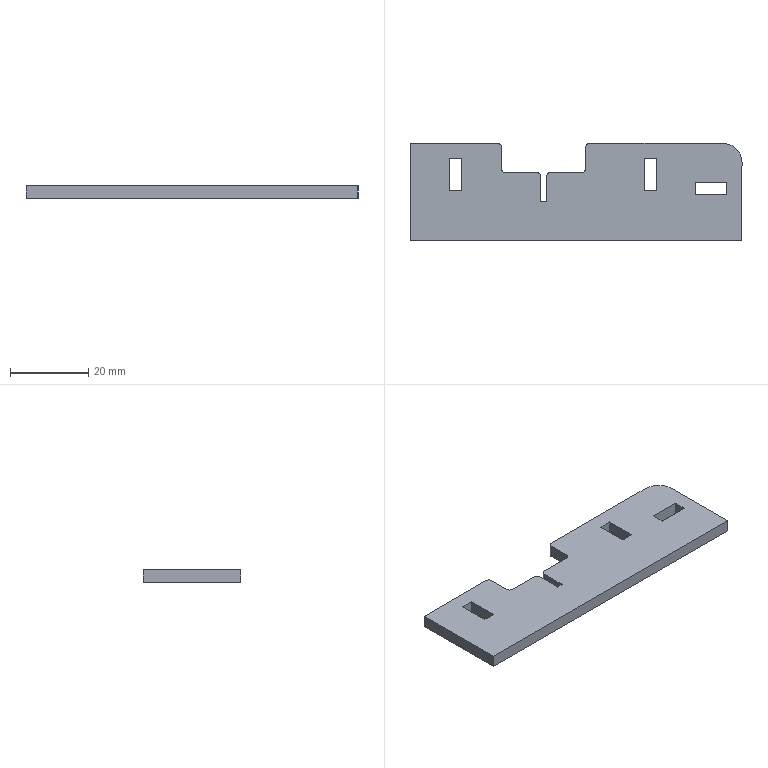Part | SolidWorks | features FlatPattern 1, SMBaseFlange 1, SheetMetal 1 | 1 solid | 33 faces | box 85 x 25 x 3.2 mm | volume 5979 mm3 | plane 26 | cylinder 7 | commonest cylinder face diameters 2 x6 10 x1
STEP:
#1=CARTESIAN_POINT('',(-85.,-5.,3.2));
#2=VERTEX_POINT('',#1);
#3=CARTESIAN_POINT('',(0.,-5.,3.2));
#4=VERTEX_POINT('',#3);
#5=CARTESIAN_POINT('',(0.,-5.,3.2));
#6=DIRECTION('',(1.,0.,0.));
#7=VECTOR('',#6,1000.);
#8=LINE('',#5,#7);
#9=EDGE_CURVE('',#2,#4,#8,.T.);
#10=ORIENTED_EDGE('',*,*,#9,.T.);
#11=CARTESIAN_POINT('',(0.,15.,3.2));
#12=VERTEX_POINT('',#11);
#13=CARTESIAN_POINT('',(0.,15.,3.2));
#14=DIRECTION('',(0.,1.,0.));
#15=VECTOR('',#14,1000.);
#16=LINE('',#13,#15);
#17=EDGE_CURVE('',#4,#12,#16,.T.);
#18=ORIENTED_EDGE('',*,*,#17,.T.);
#19=CARTESIAN_POINT('',(-5.,20.,3.2));
#20=VERTEX_POINT('',#19);
#21=CARTESIAN_POINT('',(-5.,15.,3.2));
#22=DIRECTION('',(0.,0.,1.));
#23=DIRECTION('',(-1.,0.,0.));
#24=AXIS2_PLACEMENT_3D('',#21,#22,#23);
#25=CIRCLE('',#24,5.);
#26=EDGE_CURVE('',#12,#20,#25,.T.);
#27=ORIENTED_EDGE('',*,*,#26,.T.);
#28=CARTESIAN_POINT('',(-39.,20.,3.2));
#29=VERTEX_POINT('',#28);
#30=CARTESIAN_POINT('',(-39.,20.,3.2));
#31=DIRECTION('',(-1.,0.,0.));
#32=VECTOR('',#31,1000.);
#33=LINE('',#30,#32);
#34=EDGE_CURVE('',#20,#29,#33,.T.);
#35=ORIENTED_EDGE('',*,*,#34,.T.);
#36=CARTESIAN_POINT('',(-40.,19.,3.2));
#37=VERTEX_POINT('',#36);
#38=CARTESIAN_POINT('',(-39.,19.,3.2));
#39=DIRECTION('',(0.,0.,1.));
#40=DIRECTION('',(-1.,0.,0.));
#41=AXIS2_PLACEMENT_3D('',#38,#39,#40);
#42=CIRCLE('',#41,1.);
#43=EDGE_CURVE('',#29,#37,#42,.T.);
#44=ORIENTED_EDGE('',*,*,#43,.T.);
#45=CARTESIAN_POINT('',(-40.,13.5,3.2));
#46=VERTEX_POINT('',#45);
#47=CARTESIAN_POINT('',(-40.,13.5,3.2));
#48=DIRECTION('',(0.,-1.,0.));
#49=VECTOR('',#48,1000.);
#50=LINE('',#47,#49);
#51=EDGE_CURVE('',#37,#46,#50,.T.);
#52=ORIENTED_EDGE('',*,*,#51,.T.);
#53=CARTESIAN_POINT('',(-41.,12.5,3.2));
#54=VERTEX_POINT('',#53);
#55=CARTESIAN_POINT('',(-41.,13.5,3.2));
#56=DIRECTION('',(0.,0.,-1.));
#57=DIRECTION('',(1.,0.,0.));
#58=AXIS2_PLACEMENT_3D('',#55,#56,#57);
#59=CIRCLE('',#58,1.);
#60=EDGE_CURVE('',#46,#54,#59,.T.);
#61=ORIENTED_EDGE('',*,*,#60,.T.);
#62=CARTESIAN_POINT('',(-49.,12.5,3.2));
#63=VERTEX_POINT('',#62);
#64=CARTESIAN_POINT('',(-49.,12.5,3.2));
#65=DIRECTION('',(-1.,0.,0.));
#66=VECTOR('',#65,1000.);
#67=LINE('',#64,#66);
#68=EDGE_CURVE('',#54,#63,#67,.T.);
#69=ORIENTED_EDGE('',*,*,#68,.T.);
#70=CARTESIAN_POINT('',(-50.,11.5,3.2));
#71=VERTEX_POINT('',#70);
#72=CARTESIAN_POINT('',(-49.,11.5,3.2));
#73=DIRECTION('',(0.,0.,1.));
#74=DIRECTION('',(1.,0.,0.));
#75=AXIS2_PLACEMENT_3D('',#72,#73,#74);
#76=CIRCLE('',#75,1.);
#77=EDGE_CURVE('',#63,#71,#76,.T.);
#78=ORIENTED_EDGE('',*,*,#77,.T.);
#79=CARTESIAN_POINT('',(-50.,5.,3.2));
#80=VERTEX_POINT('',#79);
#81=CARTESIAN_POINT('',(-50.,5.,3.2));
#82=DIRECTION('',(0.,-1.,0.));
#83=VECTOR('',#82,1000.);
#84=LINE('',#81,#83);
#85=EDGE_CURVE('',#71,#80,#84,.T.);
#86=ORIENTED_EDGE('',*,*,#85,.T.);
#87=CARTESIAN_POINT('',(-51.6,5.,3.2));
#88=VERTEX_POINT('',#87);
#89=CARTESIAN_POINT('',(-51.6,5.,3.2));
#90=DIRECTION('',(-1.,0.,0.));
#91=VECTOR('',#90,1000.);
#92=LINE('',#89,#91);
#93=EDGE_CURVE('',#80,#88,#92,.T.);
#94=ORIENTED_EDGE('',*,*,#93,.T.);
#95=CARTESIAN_POINT('',(-51.6,11.5,3.2));
#96=VERTEX_POINT('',#95);
#97=CARTESIAN_POINT('',(-51.6,11.5,3.2));
#98=DIRECTION('',(0.,1.,0.));
#99=VECTOR('',#98,1000.);
#100=LINE('',#97,#99);
#101=EDGE_CURVE('',#88,#96,#100,.T.);
#102=ORIENTED_EDGE('',*,*,#101,.T.);
#103=CARTESIAN_POINT('',(-52.6,12.5,3.2));
#104=VERTEX_POINT('',#103);
#105=CARTESIAN_POINT('',(-52.6,11.5,3.2));
#106=DIRECTION('',(0.,0.,1.));
#107=DIRECTION('',(-1.,0.,0.));
#108=AXIS2_PLACEMENT_3D('',#105,#106,#107);
#109=CIRCLE('',#108,1.);
#110=EDGE_CURVE('',#96,#104,#109,.T.);
#111=ORIENTED_EDGE('',*,*,#110,.T.);
#112=CARTESIAN_POINT('',(-60.6,12.5,3.2));
#113=VERTEX_POINT('',#112);
#114=CARTESIAN_POINT('',(-52.6,12.5,3.2));
#115=DIRECTION('',(-1.,0.,0.));
#116=VECTOR('',#115,1000.);
#117=LINE('',#114,#116);
#118=EDGE_CURVE('',#104,#113,#117,.T.);
#119=ORIENTED_EDGE('',*,*,#118,.T.);
#120=CARTESIAN_POINT('',(-61.6,13.5,3.2));
#121=VERTEX_POINT('',#120);
#122=CARTESIAN_POINT('',(-60.6,13.5,3.2));
#123=DIRECTION('',(0.,0.,-1.));
#124=DIRECTION('',(-1.,0.,0.));
#125=AXIS2_PLACEMENT_3D('',#122,#123,#124);
#126=CIRCLE('',#125,1.);
#127=EDGE_CURVE('',#113,#121,#126,.T.);
#128=ORIENTED_EDGE('',*,*,#127,.T.);
#129=CARTESIAN_POINT('',(-61.6,19.,3.2));
#130=VERTEX_POINT('',#129);
#131=CARTESIAN_POINT('',(-61.6,13.5,3.2));
#132=DIRECTION('',(0.,1.,0.));
#133=VECTOR('',#132,1000.);
#134=LINE('',#131,#133);
#135=EDGE_CURVE('',#121,#130,#134,.T.);
#136=ORIENTED_EDGE('',*,*,#135,.T.);
#137=CARTESIAN_POINT('',(-62.6,20.,3.2));
#138=VERTEX_POINT('',#137);
#139=CARTESIAN_POINT('',(-62.6,19.,3.2));
#140=DIRECTION('',(0.,0.,1.));
#141=DIRECTION('',(1.,0.,0.));
#142=AXIS2_PLACEMENT_3D('',#139,#140,#141);
#143=CIRCLE('',#142,1.);
#144=EDGE_CURVE('',#130,#138,#143,.T.);
#145=ORIENTED_EDGE('',*,*,#144,.T.);
#146=CARTESIAN_POINT('',(-85.,20.,3.2));
#147=VERTEX_POINT('',#146);
#148=CARTESIAN_POINT('',(-85.,20.,3.2));
#149=DIRECTION('',(-1.,0.,0.));
#150=VECTOR('',#149,1000.);
#151=LINE('',#148,#150);
#152=EDGE_CURVE('',#138,#147,#151,.T.);
#153=ORIENTED_EDGE('',*,*,#152,.T.);
#154=CARTESIAN_POINT('',(-85.,-5.,3.2));
#155=DIRECTION('',(0.,-1.,0.));
#156=VECTOR('',#155,1000.);
#157=LINE('',#154,#156);
#158=EDGE_CURVE('',#147,#2,#157,.T.);
#159=ORIENTED_EDGE('',*,*,#158,.T.);
#160=EDGE_LOOP('',(#10,#18,#27,#35,#44,#52,#61,#69,#78,#86,#94,#102,#111,#119,#128,#136,#145,#153,#159));
#161=FACE_OUTER_BOUND('',#160,.T.);
#162=CARTESIAN_POINT('',(-4.,10.,3.2));
#163=VERTEX_POINT('',#162);
#164=CARTESIAN_POINT('',(-12.,10.,3.2));
#165=VERTEX_POINT('',#164);
#166=CARTESIAN_POINT('',(-4.,10.,3.2));
#167=DIRECTION('',(-1.,0.,0.));
#168=VECTOR('',#167,1000.);
#169=LINE('',#166,#168);
#170=EDGE_CURVE('',#163,#165,#169,.T.);
#171=ORIENTED_EDGE('',*,*,#170,.F.);
#172=CARTESIAN_POINT('',(-4.,6.8,3.2));
#173=VERTEX_POINT('',#172);
#174=CARTESIAN_POINT('',(-4.,10.,3.2));
#175=DIRECTION('',(0.,1.,0.));
#176=VECTOR('',#175,1000.);
#177=LINE('',#174,#176);
#178=EDGE_CURVE('',#173,#163,#177,.T.);
#179=ORIENTED_EDGE('',*,*,#178,.F.);
#180=CARTESIAN_POINT('',(-12.,6.8,3.2));
#181=VERTEX_POINT('',#180);
#182=CARTESIAN_POINT('',(-4.,6.8,3.2));
#183=DIRECTION('',(1.,0.,0.));
#184=VECTOR('',#183,1000.);
#185=LINE('',#182,#184);
#186=EDGE_CURVE('',#181,#173,#185,.T.);
#187=ORIENTED_EDGE('',*,*,#186,.F.);
#188=CARTESIAN_POINT('',(-12.,10.,3.2));
#189=DIRECTION('',(0.,-1.,0.));
#190=VECTOR('',#189,1000.);
#191=LINE('',#188,#190);
#192=EDGE_CURVE('',#165,#181,#191,.T.);
#193=ORIENTED_EDGE('',*,*,#192,.F.);
#194=EDGE_LOOP('',(#171,#179,#187,#193));
#195=FACE_BOUND('',#194,.T.);
#196=CARTESIAN_POINT('',(-25.,8.,3.2));
#197=VERTEX_POINT('',#196);
#198=CARTESIAN_POINT('',(-21.8,8.,3.2));
#199=VERTEX_POINT('',#198);
#200=CARTESIAN_POINT('',(-25.,8.,3.2));
#201=DIRECTION('',(1.,0.,0.));
#202=VECTOR('',#201,1000.);
#203=LINE('',#200,#202);
#204=EDGE_CURVE('',#197,#199,#203,.T.);
#205=ORIENTED_EDGE('',*,*,#204,.F.);
#206=CARTESIAN_POINT('',(-25.,16.,3.2));
#207=VERTEX_POINT('',#206);
#208=CARTESIAN_POINT('',(-25.,8.,3.2));
#209=DIRECTION('',(0.,-1.,0.));
#210=VECTOR('',#209,1000.);
#211=LINE('',#208,#210);
#212=EDGE_CURVE('',#207,#197,#211,.T.);
#213=ORIENTED_EDGE('',*,*,#212,.F.);
#214=CARTESIAN_POINT('',(-21.8,16.,3.2));
#215=VERTEX_POINT('',#214);
#216=CARTESIAN_POINT('',(-25.,16.,3.2));
#217=DIRECTION('',(-1.,0.,0.));
#218=VECTOR('',#217,1000.);
#219=LINE('',#216,#218);
#220=EDGE_CURVE('',#215,#207,#219,.T.);
#221=ORIENTED_EDGE('',*,*,#220,.F.);
#222=CARTESIAN_POINT('',(-21.8,8.,3.2));
#223=DIRECTION('',(0.,1.,0.));
#224=VECTOR('',#223,1000.);
#225=LINE('',#222,#224);
#226=EDGE_CURVE('',#199,#215,#225,.T.);
#227=ORIENTED_EDGE('',*,*,#226,.F.);
#228=EDGE_LOOP('',(#205,#213,#221,#227));
#229=FACE_BOUND('',#228,.T.);
#230=CARTESIAN_POINT('',(-71.8,16.,3.2));
#231=VERTEX_POINT('',#230);
#232=CARTESIAN_POINT('',(-75.,16.,3.2));
#233=VERTEX_POINT('',#232);
#234=CARTESIAN_POINT('',(-71.8,16.,3.2));
#235=DIRECTION('',(-1.,0.,0.));
#236=VECTOR('',#235,1000.);
#237=LINE('',#234,#236);
#238=EDGE_CURVE('',#231,#233,#237,.T.);
#239=ORIENTED_EDGE('',*,*,#238,.F.);
#240=CARTESIAN_POINT('',(-71.8,8.,3.2));
#241=VERTEX_POINT('',#240);
#242=CARTESIAN_POINT('',(-71.8,8.,3.2));
#243=DIRECTION('',(0.,1.,0.));
#244=VECTOR('',#243,1000.);
#245=LINE('',#242,#244);
#246=EDGE_CURVE('',#241,#231,#245,.T.);
#247=ORIENTED_EDGE('',*,*,#246,.F.);
#248=CARTESIAN_POINT('',(-75.,8.,3.2));
#249=VERTEX_POINT('',#248);
#250=CARTESIAN_POINT('',(-71.8,8.,3.2));
#251=DIRECTION('',(1.,0.,0.));
#252=VECTOR('',#251,1000.);
#253=LINE('',#250,#252);
#254=EDGE_CURVE('',#249,#241,#253,.T.);
#255=ORIENTED_EDGE('',*,*,#254,.F.);
#256=CARTESIAN_POINT('',(-75.,8.,3.2));
#257=DIRECTION('',(0.,-1.,0.));
#258=VECTOR('',#257,1000.);
#259=LINE('',#256,#258);
#260=EDGE_CURVE('',#233,#249,#259,.T.);
#261=ORIENTED_EDGE('',*,*,#260,.F.);
#262=EDGE_LOOP('',(#239,#247,#255,#261));
#263=FACE_BOUND('',#262,.T.);
#264=CARTESIAN_POINT('',(-62.6,19.,3.2));
#265=DIRECTION('',(0.,0.,1.));
#266=DIRECTION('',(1.,0.,0.));
#267=AXIS2_PLACEMENT_3D('',#264,#265,#266);
#268=PLANE('',#267);
#269=ADVANCED_FACE('',(#161,#195,#229,#263),#268,.T.);
#270=CARTESIAN_POINT('',(-25.,16.,0.));
#271=VERTEX_POINT('',#270);
#272=CARTESIAN_POINT('',(-25.,8.,0.));
#273=VERTEX_POINT('',#272);
#274=CARTESIAN_POINT('',(-25.,8.,0.));
#275=DIRECTION('',(0.,-1.,0.));
#276=VECTOR('',#275,1000.);
#277=LINE('',#274,#276);
#278=EDGE_CURVE('',#271,#273,#277,.T.);
#279=ORIENTED_EDGE('',*,*,#278,.T.);
#280=CARTESIAN_POINT('',(-21.8,8.,0.));
#281=VERTEX_POINT('',#280);
#282=CARTESIAN_POINT('',(-25.,8.,0.));
#283=DIRECTION('',(1.,0.,0.));
#284=VECTOR('',#283,1000.);
#285=LINE('',#282,#284);
#286=EDGE_CURVE('',#273,#281,#285,.T.);
#287=ORIENTED_EDGE('',*,*,#286,.T.);
#288=CARTESIAN_POINT('',(-21.8,16.,0.));
#289=VERTEX_POINT('',#288);
#290=CARTESIAN_POINT('',(-21.8,8.,0.));
#291=DIRECTION('',(0.,1.,0.));
#292=VECTOR('',#291,1000.);
#293=LINE('',#290,#292);
#294=EDGE_CURVE('',#281,#289,#293,.T.);
#295=ORIENTED_EDGE('',*,*,#294,.T.);
#296=CARTESIAN_POINT('',(-25.,16.,0.));
#297=DIRECTION('',(-1.,0.,0.));
#298=VECTOR('',#297,1000.);
#299=LINE('',#296,#298);
#300=EDGE_CURVE('',#289,#271,#299,.T.);
#301=ORIENTED_EDGE('',*,*,#300,.T.);
#302=EDGE_LOOP('',(#279,#287,#295,#301));
#303=FACE_BOUND('',#302,.T.);
#304=CARTESIAN_POINT('',(-85.,-5.,0.));
#305=VERTEX_POINT('',#304);
#306=CARTESIAN_POINT('',(0.,-5.,0.));
#307=VERTEX_POINT('',#306);
#308=CARTESIAN_POINT('',(0.,-5.,0.));
#309=DIRECTION('',(1.,0.,0.));
#310=VECTOR('',#309,1000.);
#311=LINE('',#308,#310);
#312=EDGE_CURVE('',#305,#307,#311,.T.);
#313=ORIENTED_EDGE('',*,*,#312,.F.);
#314=CARTESIAN_POINT('',(-85.,20.,0.));
#315=VERTEX_POINT('',#314);
#316=CARTESIAN_POINT('',(-85.,-5.,0.));
#317=DIRECTION('',(0.,-1.,0.));
#318=VECTOR('',#317,1000.);
#319=LINE('',#316,#318);
#320=EDGE_CURVE('',#315,#305,#319,.T.);
#321=ORIENTED_EDGE('',*,*,#320,.F.);
#322=CARTESIAN_POINT('',(-62.6,20.,0.));
#323=VERTEX_POINT('',#322);
#324=CARTESIAN_POINT('',(-85.,20.,0.));
#325=DIRECTION('',(-1.,0.,0.));
#326=VECTOR('',#325,1000.);
#327=LINE('',#324,#326);
#328=EDGE_CURVE('',#323,#315,#327,.T.);
#329=ORIENTED_EDGE('',*,*,#328,.F.);
#330=CARTESIAN_POINT('',(-61.6,19.,0.));
#331=VERTEX_POINT('',#330);
#332=CARTESIAN_POINT('',(-62.6,19.,0.));
#333=DIRECTION('',(0.,0.,1.));
#334=DIRECTION('',(1.,0.,0.));
#335=AXIS2_PLACEMENT_3D('',#332,#333,#334);
#336=CIRCLE('',#335,1.);
#337=EDGE_CURVE('',#331,#323,#336,.T.);
#338=ORIENTED_EDGE('',*,*,#337,.F.);
#339=CARTESIAN_POINT('',(-61.6,13.5,0.));
#340=VERTEX_POINT('',#339);
#341=CARTESIAN_POINT('',(-61.6,13.5,0.));
#342=DIRECTION('',(0.,1.,0.));
#343=VECTOR('',#342,1000.);
#344=LINE('',#341,#343);
#345=EDGE_CURVE('',#340,#331,#344,.T.);
#346=ORIENTED_EDGE('',*,*,#345,.F.);
#347=CARTESIAN_POINT('',(-60.6,12.5,0.));
#348=VERTEX_POINT('',#347);
#349=CARTESIAN_POINT('',(-60.6,13.5,0.));
#350=DIRECTION('',(0.,0.,-1.));
#351=DIRECTION('',(-1.,0.,0.));
#352=AXIS2_PLACEMENT_3D('',#349,#350,#351);
#353=CIRCLE('',#352,1.);
#354=EDGE_CURVE('',#348,#340,#353,.T.);
#355=ORIENTED_EDGE('',*,*,#354,.F.);
#356=CARTESIAN_POINT('',(-52.6,12.5,0.));
#357=VERTEX_POINT('',#356);
#358=CARTESIAN_POINT('',(-52.6,12.5,0.));
#359=DIRECTION('',(-1.,0.,0.));
#360=VECTOR('',#359,1000.);
#361=LINE('',#358,#360);
#362=EDGE_CURVE('',#357,#348,#361,.T.);
#363=ORIENTED_EDGE('',*,*,#362,.F.);
#364=CARTESIAN_POINT('',(-51.6,11.5,0.));
#365=VERTEX_POINT('',#364);
#366=CARTESIAN_POINT('',(-52.6,11.5,0.));
#367=DIRECTION('',(0.,0.,1.));
#368=DIRECTION('',(-1.,0.,0.));
#369=AXIS2_PLACEMENT_3D('',#366,#367,#368);
#370=CIRCLE('',#369,1.);
#371=EDGE_CURVE('',#365,#357,#370,.T.);
#372=ORIENTED_EDGE('',*,*,#371,.F.);
#373=CARTESIAN_POINT('',(-51.6,5.,0.));
#374=VERTEX_POINT('',#373);
#375=CARTESIAN_POINT('',(-51.6,11.5,0.));
#376=DIRECTION('',(0.,1.,0.));
#377=VECTOR('',#376,1000.);
#378=LINE('',#375,#377);
#379=EDGE_CURVE('',#374,#365,#378,.T.);
#380=ORIENTED_EDGE('',*,*,#379,.F.);
#381=CARTESIAN_POINT('',(-50.,5.,0.));
#382=VERTEX_POINT('',#381);
#383=CARTESIAN_POINT('',(-51.6,5.,0.));
#384=DIRECTION('',(-1.,0.,0.));
#385=VECTOR('',#384,1000.);
#386=LINE('',#383,#385);
#387=EDGE_CURVE('',#382,#374,#386,.T.);
#388=ORIENTED_EDGE('',*,*,#387,.F.);
#389=CARTESIAN_POINT('',(-50.,11.5,0.));
#390=VERTEX_POINT('',#389);
#391=CARTESIAN_POINT('',(-50.,5.,0.));
#392=DIRECTION('',(0.,-1.,0.));
#393=VECTOR('',#392,1000.);
#394=LINE('',#391,#393);
#395=EDGE_CURVE('',#390,#382,#394,.T.);
#396=ORIENTED_EDGE('',*,*,#395,.F.);
#397=CARTESIAN_POINT('',(-49.,12.5,0.));
#398=VERTEX_POINT('',#397);
#399=CARTESIAN_POINT('',(-49.,11.5,0.));
#400=DIRECTION('',(0.,0.,1.));
#401=DIRECTION('',(1.,0.,0.));
#402=AXIS2_PLACEMENT_3D('',#399,#400,#401);
#403=CIRCLE('',#402,1.);
#404=EDGE_CURVE('',#398,#390,#403,.T.);
#405=ORIENTED_EDGE('',*,*,#404,.F.);
#406=CARTESIAN_POINT('',(-41.,12.5,0.));
#407=VERTEX_POINT('',#406);
#408=CARTESIAN_POINT('',(-49.,12.5,0.));
#409=DIRECTION('',(-1.,0.,0.));
#410=VECTOR('',#409,1000.);
#411=LINE('',#408,#410);
#412=EDGE_CURVE('',#407,#398,#411,.T.);
#413=ORIENTED_EDGE('',*,*,#412,.F.);
#414=CARTESIAN_POINT('',(-40.,13.5,0.));
#415=VERTEX_POINT('',#414);
#416=CARTESIAN_POINT('',(-41.,13.5,0.));
#417=DIRECTION('',(0.,0.,-1.));
#418=DIRECTION('',(1.,0.,0.));
#419=AXIS2_PLACEMENT_3D('',#416,#417,#418);
#420=CIRCLE('',#419,1.);
#421=EDGE_CURVE('',#415,#407,#420,.T.);
#422=ORIENTED_EDGE('',*,*,#421,.F.);
#423=CARTESIAN_POINT('',(-40.,19.,0.));
#424=VERTEX_POINT('',#423);
#425=CARTESIAN_POINT('',(-40.,13.5,0.));
#426=DIRECTION('',(0.,-1.,0.));
#427=VECTOR('',#426,1000.);
#428=LINE('',#425,#427);
#429=EDGE_CURVE('',#424,#415,#428,.T.);
#430=ORIENTED_EDGE('',*,*,#429,.F.);
#431=CARTESIAN_POINT('',(-39.,20.,0.));
#432=VERTEX_POINT('',#431);
#433=CARTESIAN_POINT('',(-39.,19.,0.));
#434=DIRECTION('',(0.,0.,1.));
#435=DIRECTION('',(-1.,0.,0.));
#436=AXIS2_PLACEMENT_3D('',#433,#434,#435);
#437=CIRCLE('',#436,1.);
#438=EDGE_CURVE('',#432,#424,#437,.T.);
#439=ORIENTED_EDGE('',*,*,#438,.F.);
#440=CARTESIAN_POINT('',(-5.,20.,0.));
#441=VERTEX_POINT('',#440);
#442=CARTESIAN_POINT('',(-39.,20.,0.));
#443=DIRECTION('',(-1.,0.,0.));
#444=VECTOR('',#443,1000.);
#445=LINE('',#442,#444);
#446=EDGE_CURVE('',#441,#432,#445,.T.);
#447=ORIENTED_EDGE('',*,*,#446,.F.);
#448=CARTESIAN_POINT('',(0.,15.,0.));
#449=VERTEX_POINT('',#448);
#450=CARTESIAN_POINT('',(-5.,15.,0.));
#451=DIRECTION('',(0.,0.,1.));
#452=DIRECTION('',(-1.,0.,0.));
#453=AXIS2_PLACEMENT_3D('',#450,#451,#452);
#454=CIRCLE('',#453,5.);
#455=EDGE_CURVE('',#449,#441,#454,.T.);
#456=ORIENTED_EDGE('',*,*,#455,.F.);
#457=CARTESIAN_POINT('',(0.,15.,0.));
#458=DIRECTION('',(0.,1.,0.));
#459=VECTOR('',#458,1000.);
#460=LINE('',#457,#459);
#461=EDGE_CURVE('',#307,#449,#460,.T.);
#462=ORIENTED_EDGE('',*,*,#461,.F.);
#463=EDGE_LOOP('',(#313,#321,#329,#338,#346,#355,#363,#372,#380,#388,#396,#405,#413,#422,#430,#439,#447,#456,#462));
#464=FACE_OUTER_BOUND('',#463,.T.);
#465=CARTESIAN_POINT('',(-4.,6.8,0.));
#466=VERTEX_POINT('',#465);
#467=CARTESIAN_POINT('',(-4.,10.,0.));
#468=VERTEX_POINT('',#467);
#469=CARTESIAN_POINT('',(-4.,10.,0.));
#470=DIRECTION('',(0.,1.,0.));
#471=VECTOR('',#470,1000.);
#472=LINE('',#469,#471);
#473=EDGE_CURVE('',#466,#468,#472,.T.);
#474=ORIENTED_EDGE('',*,*,#473,.T.);
#475=CARTESIAN_POINT('',(-12.,10.,0.));
#476=VERTEX_POINT('',#475);
#477=CARTESIAN_POINT('',(-4.,10.,0.));
#478=DIRECTION('',(-1.,0.,0.));
#479=VECTOR('',#478,1000.);
#480=LINE('',#477,#479);
#481=EDGE_CURVE('',#468,#476,#480,.T.);
#482=ORIENTED_EDGE('',*,*,#481,.T.);
#483=CARTESIAN_POINT('',(-12.,6.8,0.));
#484=VERTEX_POINT('',#483);
#485=CARTESIAN_POINT('',(-12.,10.,0.));
#486=DIRECTION('',(0.,-1.,0.));
#487=VECTOR('',#486,1000.);
#488=LINE('',#485,#487);
#489=EDGE_CURVE('',#476,#484,#488,.T.);
#490=ORIENTED_EDGE('',*,*,#489,.T.);
#491=CARTESIAN_POINT('',(-4.,6.8,0.));
#492=DIRECTION('',(1.,0.,0.));
#493=VECTOR('',#492,1000.);
#494=LINE('',#491,#493);
#495=EDGE_CURVE('',#484,#466,#494,.T.);
#496=ORIENTED_EDGE('',*,*,#495,.T.);
#497=EDGE_LOOP('',(#474,#482,#490,#496));
#498=FACE_BOUND('',#497,.T.);
#499=CARTESIAN_POINT('',(-71.8,8.,0.));
#500=VERTEX_POINT('',#499);
#501=CARTESIAN_POINT('',(-71.8,16.,0.));
#502=VERTEX_POINT('',#501);
#503=CARTESIAN_POINT('',(-71.8,8.,0.));
#504=DIRECTION('',(0.,1.,0.));
#505=VECTOR('',#504,1000.);
#506=LINE('',#503,#505);
#507=EDGE_CURVE('',#500,#502,#506,.T.);
#508=ORIENTED_EDGE('',*,*,#507,.T.);
#509=CARTESIAN_POINT('',(-75.,16.,0.));
#510=VERTEX_POINT('',#509);
#511=CARTESIAN_POINT('',(-71.8,16.,0.));
#512=DIRECTION('',(-1.,0.,0.));
#513=VECTOR('',#512,1000.);
#514=LINE('',#511,#513);
#515=EDGE_CURVE('',#502,#510,#514,.T.);
#516=ORIENTED_EDGE('',*,*,#515,.T.);
#517=CARTESIAN_POINT('',(-75.,8.,0.));
#518=VERTEX_POINT('',#517);
#519=CARTESIAN_POINT('',(-75.,8.,0.));
#520=DIRECTION('',(0.,-1.,0.));
#521=VECTOR('',#520,1000.);
#522=LINE('',#519,#521);
#523=EDGE_CURVE('',#510,#518,#522,.T.);
#524=ORIENTED_EDGE('',*,*,#523,.T.);
#525=CARTESIAN_POINT('',(-71.8,8.,0.));
#526=DIRECTION('',(1.,0.,0.));
#527=VECTOR('',#526,1000.);
#528=LINE('',#525,#527);
#529=EDGE_CURVE('',#518,#500,#528,.T.);
#530=ORIENTED_EDGE('',*,*,#529,.T.);
#531=EDGE_LOOP('',(#508,#516,#524,#530));
#532=FACE_BOUND('',#531,.T.);
#533=CARTESIAN_POINT('',(-62.6,19.,0.));
#534=DIRECTION('',(0.,0.,1.));
#535=DIRECTION('',(1.,0.,0.));
#536=AXIS2_PLACEMENT_3D('',#533,#534,#535);
#537=PLANE('',#536);
#538=ADVANCED_FACE('',(#303,#464,#498,#532),#537,.F.);
#539=ORIENTED_EDGE('',*,*,#312,.T.);
#540=CARTESIAN_POINT('',(0.,-5.,3.2));
#541=DIRECTION('',(0.,0.,-1.));
#542=VECTOR('',#541,1000.);
#543=LINE('',#540,#542);
#544=EDGE_CURVE('',#4,#307,#543,.T.);
#545=ORIENTED_EDGE('',*,*,#544,.F.);
#546=ORIENTED_EDGE('',*,*,#9,.F.);
#547=CARTESIAN_POINT('',(-85.,-5.,3.2));
#548=DIRECTION('',(0.,0.,-1.));
#549=VECTOR('',#548,1000.);
#550=LINE('',#547,#549);
#551=EDGE_CURVE('',#2,#305,#550,.T.);
#552=ORIENTED_EDGE('',*,*,#551,.T.);
#553=EDGE_LOOP('',(#539,#545,#546,#552));
#554=FACE_OUTER_BOUND('',#553,.T.);
#555=CARTESIAN_POINT('',(0.,-5.,3.2));
#556=DIRECTION('',(0.,1.,0.));
#557=DIRECTION('',(-1.,0.,0.));
#558=AXIS2_PLACEMENT_3D('',#555,#556,#557);
#559=PLANE('',#558);
#560=ADVANCED_FACE('',(#554),#559,.F.);
#561=ORIENTED_EDGE('',*,*,#461,.T.);
#562=CARTESIAN_POINT('',(0.,15.,3.2));
#563=DIRECTION('',(0.,0.,-1.));
#564=VECTOR('',#563,1000.);
#565=LINE('',#562,#564);
#566=EDGE_CURVE('',#12,#449,#565,.T.);
#567=ORIENTED_EDGE('',*,*,#566,.F.);
#568=ORIENTED_EDGE('',*,*,#17,.F.);
#569=ORIENTED_EDGE('',*,*,#544,.T.);
#570=EDGE_LOOP('',(#561,#567,#568,#569));
#571=FACE_OUTER_BOUND('',#570,.T.);
#572=CARTESIAN_POINT('',(0.,15.,3.2));
#573=DIRECTION('',(-1.,0.,0.));
#574=DIRECTION('',(0.,-1.,0.));
#575=AXIS2_PLACEMENT_3D('',#572,#573,#574);
#576=PLANE('',#575);
#577=ADVANCED_FACE('',(#571),#576,.F.);
#578=ORIENTED_EDGE('',*,*,#455,.T.);
#579=CARTESIAN_POINT('',(-5.,20.,3.2));
#580=DIRECTION('',(0.,0.,-1.));
#581=VECTOR('',#580,1000.);
#582=LINE('',#579,#581);
#583=EDGE_CURVE('',#20,#441,#582,.T.);
#584=ORIENTED_EDGE('',*,*,#583,.F.);
#585=ORIENTED_EDGE('',*,*,#26,.F.);
#586=ORIENTED_EDGE('',*,*,#566,.T.);
#587=EDGE_LOOP('',(#578,#584,#585,#586));
#588=FACE_OUTER_BOUND('',#587,.T.);
#589=CARTESIAN_POINT('',(-5.,15.,3.2));
#590=DIRECTION('',(0.,0.,-1.));
#591=DIRECTION('',(-1.,0.,0.));
#592=AXIS2_PLACEMENT_3D('',#589,#590,#591);
#593=CYLINDRICAL_SURFACE('',#592,5.);
#594=ADVANCED_FACE('',(#588),#593,.T.);
#595=ORIENTED_EDGE('',*,*,#446,.T.);
#596=CARTESIAN_POINT('',(-39.,20.,3.2));
#597=DIRECTION('',(0.,0.,-1.));
#598=VECTOR('',#597,1000.);
#599=LINE('',#596,#598);
#600=EDGE_CURVE('',#29,#432,#599,.T.);
#601=ORIENTED_EDGE('',*,*,#600,.F.);
#602=ORIENTED_EDGE('',*,*,#34,.F.);
#603=ORIENTED_EDGE('',*,*,#583,.T.);
#604=EDGE_LOOP('',(#595,#601,#602,#603));
#605=FACE_OUTER_BOUND('',#604,.T.);
#606=CARTESIAN_POINT('',(-39.,20.,3.2));
#607=DIRECTION('',(0.,-1.,0.));
#608=DIRECTION('',(1.,0.,0.));
#609=AXIS2_PLACEMENT_3D('',#606,#607,#608);
#610=PLANE('',#609);
#611=ADVANCED_FACE('',(#605),#610,.F.);
#612=ORIENTED_EDGE('',*,*,#438,.T.);
#613=CARTESIAN_POINT('',(-40.,19.,3.2));
#614=DIRECTION('',(0.,0.,-1.));
#615=VECTOR('',#614,1000.);
#616=LINE('',#613,#615);
#617=EDGE_CURVE('',#37,#424,#616,.T.);
#618=ORIENTED_EDGE('',*,*,#617,.F.);
#619=ORIENTED_EDGE('',*,*,#43,.F.);
#620=ORIENTED_EDGE('',*,*,#600,.T.);
#621=EDGE_LOOP('',(#612,#618,#619,#620));
#622=FACE_OUTER_BOUND('',#621,.T.);
#623=CARTESIAN_POINT('',(-39.,19.,3.2));
#624=DIRECTION('',(0.,0.,-1.));
#625=DIRECTION('',(-1.,0.,0.));
#626=AXIS2_PLACEMENT_3D('',#623,#624,#625);
#627=CYLINDRICAL_SURFACE('',#626,1.);
#628=ADVANCED_FACE('',(#622),#627,.T.);
#629=ORIENTED_EDGE('',*,*,#429,.T.);
#630=CARTESIAN_POINT('',(-40.,13.5,3.2));
#631=DIRECTION('',(0.,0.,-1.));
#632=VECTOR('',#631,1000.);
#633=LINE('',#630,#632);
#634=EDGE_CURVE('',#46,#415,#633,.T.);
#635=ORIENTED_EDGE('',*,*,#634,.F.);
#636=ORIENTED_EDGE('',*,*,#51,.F.);
#637=ORIENTED_EDGE('',*,*,#617,.T.);
#638=EDGE_LOOP('',(#629,#635,#636,#637));
#639=FACE_OUTER_BOUND('',#638,.T.);
#640=CARTESIAN_POINT('',(-40.,13.5,3.2));
#641=DIRECTION('',(1.,0.,0.));
#642=DIRECTION('',(0.,0.,-1.));
#643=AXIS2_PLACEMENT_3D('',#640,#641,#642);
#644=PLANE('',#643);
#645=ADVANCED_FACE('',(#639),#644,.F.);
#646=ORIENTED_EDGE('',*,*,#421,.T.);
#647=CARTESIAN_POINT('',(-41.,12.5,3.2));
#648=DIRECTION('',(0.,0.,-1.));
#649=VECTOR('',#648,1000.);
#650=LINE('',#647,#649);
#651=EDGE_CURVE('',#54,#407,#650,.T.);
#652=ORIENTED_EDGE('',*,*,#651,.F.);
#653=ORIENTED_EDGE('',*,*,#60,.F.);
#654=ORIENTED_EDGE('',*,*,#634,.T.);
#655=EDGE_LOOP('',(#646,#652,#653,#654));
#656=FACE_OUTER_BOUND('',#655,.T.);
#657=CARTESIAN_POINT('',(-41.,13.5,3.2));
#658=DIRECTION('',(0.,0.,-1.));
#659=DIRECTION('',(-1.,0.,0.));
#660=AXIS2_PLACEMENT_3D('',#657,#658,#659);
#661=CYLINDRICAL_SURFACE('',#660,1.);
#662=ADVANCED_FACE('',(#656),#661,.F.);
#663=ORIENTED_EDGE('',*,*,#412,.T.);
#664=CARTESIAN_POINT('',(-49.,12.5,3.2));
#665=DIRECTION('',(0.,0.,-1.));
#666=VECTOR('',#665,1000.);
#667=LINE('',#664,#666);
#668=EDGE_CURVE('',#63,#398,#667,.T.);
#669=ORIENTED_EDGE('',*,*,#668,.F.);
#670=ORIENTED_EDGE('',*,*,#68,.F.);
#671=ORIENTED_EDGE('',*,*,#651,.T.);
#672=EDGE_LOOP('',(#663,#669,#670,#671));
#673=FACE_OUTER_BOUND('',#672,.T.);
#674=CARTESIAN_POINT('',(-49.,12.5,3.2));
#675=DIRECTION('',(0.,-1.,0.));
#676=DIRECTION('',(0.,0.,-1.));
#677=AXIS2_PLACEMENT_3D('',#674,#675,#676);
#678=PLANE('',#677);
#679=ADVANCED_FACE('',(#673),#678,.F.);
#680=ORIENTED_EDGE('',*,*,#404,.T.);
#681=CARTESIAN_POINT('',(-50.,11.5,3.2));
#682=DIRECTION('',(0.,0.,-1.));
#683=VECTOR('',#682,1000.);
#684=LINE('',#681,#683);
#685=EDGE_CURVE('',#71,#390,#684,.T.);
#686=ORIENTED_EDGE('',*,*,#685,.F.);
#687=ORIENTED_EDGE('',*,*,#77,.F.);
#688=ORIENTED_EDGE('',*,*,#668,.T.);
#689=EDGE_LOOP('',(#680,#686,#687,#688));
#690=FACE_OUTER_BOUND('',#689,.T.);
#691=CARTESIAN_POINT('',(-49.,11.5,3.2));
#692=DIRECTION('',(0.,0.,-1.));
#693=DIRECTION('',(-1.,0.,0.));
#694=AXIS2_PLACEMENT_3D('',#691,#692,#693);
#695=CYLINDRICAL_SURFACE('',#694,1.);
#696=ADVANCED_FACE('',(#690),#695,.T.);
#697=ORIENTED_EDGE('',*,*,#395,.T.);
#698=CARTESIAN_POINT('',(-50.,5.,3.2));
#699=DIRECTION('',(0.,0.,-1.));
#700=VECTOR('',#699,1000.);
#701=LINE('',#698,#700);
#702=EDGE_CURVE('',#80,#382,#701,.T.);
#703=ORIENTED_EDGE('',*,*,#702,.F.);
#704=ORIENTED_EDGE('',*,*,#85,.F.);
#705=ORIENTED_EDGE('',*,*,#685,.T.);
#706=EDGE_LOOP('',(#697,#703,#704,#705));
#707=FACE_OUTER_BOUND('',#706,.T.);
#708=CARTESIAN_POINT('',(-50.,5.,3.2));
#709=DIRECTION('',(1.,0.,0.));
#710=DIRECTION('',(0.,0.,-1.));
#711=AXIS2_PLACEMENT_3D('',#708,#709,#710);
#712=PLANE('',#711);
#713=ADVANCED_FACE('',(#707),#712,.F.);
#714=ORIENTED_EDGE('',*,*,#387,.T.);
#715=CARTESIAN_POINT('',(-51.6,5.,3.2));
#716=DIRECTION('',(0.,0.,-1.));
#717=VECTOR('',#716,1000.);
#718=LINE('',#715,#717);
#719=EDGE_CURVE('',#88,#374,#718,.T.);
#720=ORIENTED_EDGE('',*,*,#719,.F.);
#721=ORIENTED_EDGE('',*,*,#93,.F.);
#722=ORIENTED_EDGE('',*,*,#702,.T.);
#723=EDGE_LOOP('',(#714,#720,#721,#722));
#724=FACE_OUTER_BOUND('',#723,.T.);
#725=CARTESIAN_POINT('',(-51.6,5.,3.2));
#726=DIRECTION('',(0.,-1.,0.));
#727=DIRECTION('',(1.,0.,0.));
#728=AXIS2_PLACEMENT_3D('',#725,#726,#727);
#729=PLANE('',#728);
#730=ADVANCED_FACE('',(#724),#729,.F.);
#731=ORIENTED_EDGE('',*,*,#379,.T.);
#732=CARTESIAN_POINT('',(-51.6,11.5,3.2));
#733=DIRECTION('',(0.,0.,-1.));
#734=VECTOR('',#733,1000.);
#735=LINE('',#732,#734);
#736=EDGE_CURVE('',#96,#365,#735,.T.);
#737=ORIENTED_EDGE('',*,*,#736,.F.);
#738=ORIENTED_EDGE('',*,*,#101,.F.);
#739=ORIENTED_EDGE('',*,*,#719,.T.);
#740=EDGE_LOOP('',(#731,#737,#738,#739));
#741=FACE_OUTER_BOUND('',#740,.T.);
#742=CARTESIAN_POINT('',(-51.6,11.5,3.2));
#743=DIRECTION('',(-1.,0.,0.));
#744=DIRECTION('',(0.,0.,1.));
#745=AXIS2_PLACEMENT_3D('',#742,#743,#744);
#746=PLANE('',#745);
#747=ADVANCED_FACE('',(#741),#746,.F.);
#748=ORIENTED_EDGE('',*,*,#371,.T.);
#749=CARTESIAN_POINT('',(-52.6,12.5,3.2));
#750=DIRECTION('',(0.,0.,-1.));
#751=VECTOR('',#750,1000.);
#752=LINE('',#749,#751);
#753=EDGE_CURVE('',#104,#357,#752,.T.);
#754=ORIENTED_EDGE('',*,*,#753,.F.);
#755=ORIENTED_EDGE('',*,*,#110,.F.);
#756=ORIENTED_EDGE('',*,*,#736,.T.);
#757=EDGE_LOOP('',(#748,#754,#755,#756));
#758=FACE_OUTER_BOUND('',#757,.T.);
#759=CARTESIAN_POINT('',(-52.6,11.5,3.2));
#760=DIRECTION('',(0.,0.,-1.));
#761=DIRECTION('',(-1.,0.,0.));
#762=AXIS2_PLACEMENT_3D('',#759,#760,#761);
#763=CYLINDRICAL_SURFACE('',#762,1.);
#764=ADVANCED_FACE('',(#758),#763,.T.);
#765=ORIENTED_EDGE('',*,*,#362,.T.);
#766=CARTESIAN_POINT('',(-60.6,12.5,3.2));
#767=DIRECTION('',(0.,0.,-1.));
#768=VECTOR('',#767,1000.);
#769=LINE('',#766,#768);
#770=EDGE_CURVE('',#113,#348,#769,.T.);
#771=ORIENTED_EDGE('',*,*,#770,.F.);
#772=ORIENTED_EDGE('',*,*,#118,.F.);
#773=ORIENTED_EDGE('',*,*,#753,.T.);
#774=EDGE_LOOP('',(#765,#771,#772,#773));
#775=FACE_OUTER_BOUND('',#774,.T.);
#776=CARTESIAN_POINT('',(-52.6,12.5,3.2));
#777=DIRECTION('',(0.,-1.,0.));
#778=DIRECTION('',(0.,0.,-1.));
#779=AXIS2_PLACEMENT_3D('',#776,#777,#778);
#780=PLANE('',#779);
#781=ADVANCED_FACE('',(#775),#780,.F.);
#782=ORIENTED_EDGE('',*,*,#354,.T.);
#783=CARTESIAN_POINT('',(-61.6,13.5,3.2));
#784=DIRECTION('',(0.,0.,-1.));
#785=VECTOR('',#784,1000.);
#786=LINE('',#783,#785);
#787=EDGE_CURVE('',#121,#340,#786,.T.);
#788=ORIENTED_EDGE('',*,*,#787,.F.);
#789=ORIENTED_EDGE('',*,*,#127,.F.);
#790=ORIENTED_EDGE('',*,*,#770,.T.);
#791=EDGE_LOOP('',(#782,#788,#789,#790));
#792=FACE_OUTER_BOUND('',#791,.T.);
#793=CARTESIAN_POINT('',(-60.6,13.5,3.2));
#794=DIRECTION('',(0.,0.,-1.));
#795=DIRECTION('',(-1.,0.,0.));
#796=AXIS2_PLACEMENT_3D('',#793,#794,#795);
#797=CYLINDRICAL_SURFACE('',#796,1.);
#798=ADVANCED_FACE('',(#792),#797,.F.);
#799=ORIENTED_EDGE('',*,*,#345,.T.);
#800=CARTESIAN_POINT('',(-61.6,19.,3.2));
#801=DIRECTION('',(0.,0.,-1.));
#802=VECTOR('',#801,1000.);
#803=LINE('',#800,#802);
#804=EDGE_CURVE('',#130,#331,#803,.T.);
#805=ORIENTED_EDGE('',*,*,#804,.F.);
#806=ORIENTED_EDGE('',*,*,#135,.F.);
#807=ORIENTED_EDGE('',*,*,#787,.T.);
#808=EDGE_LOOP('',(#799,#805,#806,#807));
#809=FACE_OUTER_BOUND('',#808,.T.);
#810=CARTESIAN_POINT('',(-61.6,13.5,3.2));
#811=DIRECTION('',(-1.,0.,0.));
#812=DIRECTION('',(0.,-1.,0.));
#813=AXIS2_PLACEMENT_3D('',#810,#811,#812);
#814=PLANE('',#813);
#815=ADVANCED_FACE('',(#809),#814,.F.);
#816=ORIENTED_EDGE('',*,*,#337,.T.);
#817=CARTESIAN_POINT('',(-62.6,20.,3.2));
#818=DIRECTION('',(0.,0.,-1.));
#819=VECTOR('',#818,1000.);
#820=LINE('',#817,#819);
#821=EDGE_CURVE('',#138,#323,#820,.T.);
#822=ORIENTED_EDGE('',*,*,#821,.F.);
#823=ORIENTED_EDGE('',*,*,#144,.F.);
#824=ORIENTED_EDGE('',*,*,#804,.T.);
#825=EDGE_LOOP('',(#816,#822,#823,#824));
#826=FACE_OUTER_BOUND('',#825,.T.);
#827=CARTESIAN_POINT('',(-62.6,19.,3.2));
#828=DIRECTION('',(0.,0.,-1.));
#829=DIRECTION('',(-1.,0.,0.));
#830=AXIS2_PLACEMENT_3D('',#827,#828,#829);
#831=CYLINDRICAL_SURFACE('',#830,1.);
#832=ADVANCED_FACE('',(#826),#831,.T.);
#833=ORIENTED_EDGE('',*,*,#328,.T.);
#834=CARTESIAN_POINT('',(-85.,20.,3.2));
#835=DIRECTION('',(0.,0.,-1.));
#836=VECTOR('',#835,1000.);
#837=LINE('',#834,#836);
#838=EDGE_CURVE('',#147,#315,#837,.T.);
#839=ORIENTED_EDGE('',*,*,#838,.F.);
#840=ORIENTED_EDGE('',*,*,#152,.F.);
#841=ORIENTED_EDGE('',*,*,#821,.T.);
#842=EDGE_LOOP('',(#833,#839,#840,#841));
#843=FACE_OUTER_BOUND('',#842,.T.);
#844=CARTESIAN_POINT('',(-85.,20.,3.2));
#845=DIRECTION('',(0.,-1.,0.));
#846=DIRECTION('',(1.,0.,0.));
#847=AXIS2_PLACEMENT_3D('',#844,#845,#846);
#848=PLANE('',#847);
#849=ADVANCED_FACE('',(#843),#848,.F.);
#850=ORIENTED_EDGE('',*,*,#320,.T.);
#851=ORIENTED_EDGE('',*,*,#551,.F.);
#852=ORIENTED_EDGE('',*,*,#158,.F.);
#853=ORIENTED_EDGE('',*,*,#838,.T.);
#854=EDGE_LOOP('',(#850,#851,#852,#853));
#855=FACE_OUTER_BOUND('',#854,.T.);
#856=CARTESIAN_POINT('',(-85.,-5.,3.2));
#857=DIRECTION('',(1.,0.,0.));
#858=DIRECTION('',(0.,1.,0.));
#859=AXIS2_PLACEMENT_3D('',#856,#857,#858);
#860=PLANE('',#859);
#861=ADVANCED_FACE('',(#855),#860,.F.);
#862=ORIENTED_EDGE('',*,*,#473,.F.);
#863=CARTESIAN_POINT('',(-4.,6.8,3.2));
#864=DIRECTION('',(0.,0.,-1.));
#865=VECTOR('',#864,1000.);
#866=LINE('',#863,#865);
#867=EDGE_CURVE('',#173,#466,#866,.T.);
#868=ORIENTED_EDGE('',*,*,#867,.F.);
#869=ORIENTED_EDGE('',*,*,#178,.T.);
#870=CARTESIAN_POINT('',(-4.,10.,3.2));
#871=DIRECTION('',(0.,0.,-1.));
#872=VECTOR('',#871,1000.);
#873=LINE('',#870,#872);
#874=EDGE_CURVE('',#163,#468,#873,.T.);
#875=ORIENTED_EDGE('',*,*,#874,.T.);
#876=EDGE_LOOP('',(#862,#868,#869,#875));
#877=FACE_OUTER_BOUND('',#876,.T.);
#878=CARTESIAN_POINT('',(-4.,10.,3.2));
#879=DIRECTION('',(-1.,0.,0.));
#880=DIRECTION('',(0.,0.,1.));
#881=AXIS2_PLACEMENT_3D('',#878,#879,#880);
#882=PLANE('',#881);
#883=ADVANCED_FACE('',(#877),#882,.T.);
#884=ORIENTED_EDGE('',*,*,#481,.F.);
#885=ORIENTED_EDGE('',*,*,#874,.F.);
#886=ORIENTED_EDGE('',*,*,#170,.T.);
#887=CARTESIAN_POINT('',(-12.,10.,3.2));
#888=DIRECTION('',(0.,0.,-1.));
#889=VECTOR('',#888,1000.);
#890=LINE('',#887,#889);
#891=EDGE_CURVE('',#165,#476,#890,.T.);
#892=ORIENTED_EDGE('',*,*,#891,.T.);
#893=EDGE_LOOP('',(#884,#885,#886,#892));
#894=FACE_OUTER_BOUND('',#893,.T.);
#895=CARTESIAN_POINT('',(-4.,10.,3.2));
#896=DIRECTION('',(0.,-1.,0.));
#897=DIRECTION('',(0.,0.,-1.));
#898=AXIS2_PLACEMENT_3D('',#895,#896,#897);
#899=PLANE('',#898);
#900=ADVANCED_FACE('',(#894),#899,.T.);
#901=ORIENTED_EDGE('',*,*,#489,.F.);
#902=ORIENTED_EDGE('',*,*,#891,.F.);
#903=ORIENTED_EDGE('',*,*,#192,.T.);
#904=CARTESIAN_POINT('',(-12.,6.8,3.2));
#905=DIRECTION('',(0.,0.,-1.));
#906=VECTOR('',#905,1000.);
#907=LINE('',#904,#906);
#908=EDGE_CURVE('',#181,#484,#907,.T.);
#909=ORIENTED_EDGE('',*,*,#908,.T.);
#910=EDGE_LOOP('',(#901,#902,#903,#909));
#911=FACE_OUTER_BOUND('',#910,.T.);
#912=CARTESIAN_POINT('',(-12.,10.,3.2));
#913=DIRECTION('',(1.,0.,0.));
#914=DIRECTION('',(0.,0.,-1.));
#915=AXIS2_PLACEMENT_3D('',#912,#913,#914);
#916=PLANE('',#915);
#917=ADVANCED_FACE('',(#911),#916,.T.);
#918=ORIENTED_EDGE('',*,*,#495,.F.);
#919=ORIENTED_EDGE('',*,*,#908,.F.);
#920=ORIENTED_EDGE('',*,*,#186,.T.);
#921=ORIENTED_EDGE('',*,*,#867,.T.);
#922=EDGE_LOOP('',(#918,#919,#920,#921));
#923=FACE_OUTER_BOUND('',#922,.T.);
#924=CARTESIAN_POINT('',(-4.,6.8,3.2));
#925=DIRECTION('',(0.,1.,0.));
#926=DIRECTION('',(0.,0.,1.));
#927=AXIS2_PLACEMENT_3D('',#924,#925,#926);
#928=PLANE('',#927);
#929=ADVANCED_FACE('',(#923),#928,.T.);
#930=ORIENTED_EDGE('',*,*,#278,.F.);
#931=CARTESIAN_POINT('',(-25.,16.,3.2));
#932=DIRECTION('',(0.,0.,-1.));
#933=VECTOR('',#932,1000.);
#934=LINE('',#931,#933);
#935=EDGE_CURVE('',#207,#271,#934,.T.);
#936=ORIENTED_EDGE('',*,*,#935,.F.);
#937=ORIENTED_EDGE('',*,*,#212,.T.);
#938=CARTESIAN_POINT('',(-25.,8.,3.2));
#939=DIRECTION('',(0.,0.,-1.));
#940=VECTOR('',#939,1000.);
#941=LINE('',#938,#940);
#942=EDGE_CURVE('',#197,#273,#941,.T.);
#943=ORIENTED_EDGE('',*,*,#942,.T.);
#944=EDGE_LOOP('',(#930,#936,#937,#943));
#945=FACE_OUTER_BOUND('',#944,.T.);
#946=CARTESIAN_POINT('',(-25.,8.,3.2));
#947=DIRECTION('',(1.,0.,0.));
#948=DIRECTION('',(0.,0.,-1.));
#949=AXIS2_PLACEMENT_3D('',#946,#947,#948);
#950=PLANE('',#949);
#951=ADVANCED_FACE('',(#945),#950,.T.);
#952=ORIENTED_EDGE('',*,*,#286,.F.);
#953=ORIENTED_EDGE('',*,*,#942,.F.);
#954=ORIENTED_EDGE('',*,*,#204,.T.);
#955=CARTESIAN_POINT('',(-21.8,8.,3.2));
#956=DIRECTION('',(0.,0.,-1.));
#957=VECTOR('',#956,1000.);
#958=LINE('',#955,#957);
#959=EDGE_CURVE('',#199,#281,#958,.T.);
#960=ORIENTED_EDGE('',*,*,#959,.T.);
#961=EDGE_LOOP('',(#952,#953,#954,#960));
#962=FACE_OUTER_BOUND('',#961,.T.);
#963=CARTESIAN_POINT('',(-25.,8.,3.2));
#964=DIRECTION('',(0.,1.,0.));
#965=DIRECTION('',(0.,0.,1.));
#966=AXIS2_PLACEMENT_3D('',#963,#964,#965);
#967=PLANE('',#966);
#968=ADVANCED_FACE('',(#962),#967,.T.);
#969=ORIENTED_EDGE('',*,*,#294,.F.);
#970=ORIENTED_EDGE('',*,*,#959,.F.);
#971=ORIENTED_EDGE('',*,*,#226,.T.);
#972=CARTESIAN_POINT('',(-21.8,16.,3.2));
#973=DIRECTION('',(0.,0.,-1.));
#974=VECTOR('',#973,1000.);
#975=LINE('',#972,#974);
#976=EDGE_CURVE('',#215,#289,#975,.T.);
#977=ORIENTED_EDGE('',*,*,#976,.T.);
#978=EDGE_LOOP('',(#969,#970,#971,#977));
#979=FACE_OUTER_BOUND('',#978,.T.);
#980=CARTESIAN_POINT('',(-21.8,8.,3.2));
#981=DIRECTION('',(-1.,0.,0.));
#982=DIRECTION('',(0.,0.,1.));
#983=AXIS2_PLACEMENT_3D('',#980,#981,#982);
#984=PLANE('',#983);
#985=ADVANCED_FACE('',(#979),#984,.T.);
#986=ORIENTED_EDGE('',*,*,#300,.F.);
#987=ORIENTED_EDGE('',*,*,#976,.F.);
#988=ORIENTED_EDGE('',*,*,#220,.T.);
#989=ORIENTED_EDGE('',*,*,#935,.T.);
#990=EDGE_LOOP('',(#986,#987,#988,#989));
#991=FACE_OUTER_BOUND('',#990,.T.);
#992=CARTESIAN_POINT('',(-25.,16.,3.2));
#993=DIRECTION('',(0.,-1.,0.));
#994=DIRECTION('',(0.,0.,-1.));
#995=AXIS2_PLACEMENT_3D('',#992,#993,#994);
#996=PLANE('',#995);
#997=ADVANCED_FACE('',(#991),#996,.T.);
#998=ORIENTED_EDGE('',*,*,#507,.F.);
#999=CARTESIAN_POINT('',(-71.8,8.,3.2));
#1000=DIRECTION('',(0.,0.,-1.));
#1001=VECTOR('',#1000,1000.);
#1002=LINE('',#999,#1001);
#1003=EDGE_CURVE('',#241,#500,#1002,.T.);
#1004=ORIENTED_EDGE('',*,*,#1003,.F.);
#1005=ORIENTED_EDGE('',*,*,#246,.T.);
#1006=CARTESIAN_POINT('',(-71.8,16.,3.2));
#1007=DIRECTION('',(0.,0.,-1.));
#1008=VECTOR('',#1007,1000.);
#1009=LINE('',#1006,#1008);
#1010=EDGE_CURVE('',#231,#502,#1009,.T.);
#1011=ORIENTED_EDGE('',*,*,#1010,.T.);
#1012=EDGE_LOOP('',(#998,#1004,#1005,#1011));
#1013=FACE_OUTER_BOUND('',#1012,.T.);
#1014=CARTESIAN_POINT('',(-71.8,8.,3.2));
#1015=DIRECTION('',(-1.,0.,0.));
#1016=DIRECTION('',(0.,0.,1.));
#1017=AXIS2_PLACEMENT_3D('',#1014,#1015,#1016);
#1018=PLANE('',#1017);
#1019=ADVANCED_FACE('',(#1013),#1018,.T.);
#1020=ORIENTED_EDGE('',*,*,#515,.F.);
#1021=ORIENTED_EDGE('',*,*,#1010,.F.);
#1022=ORIENTED_EDGE('',*,*,#238,.T.);
#1023=CARTESIAN_POINT('',(-75.,16.,3.2));
#1024=DIRECTION('',(0.,0.,-1.));
#1025=VECTOR('',#1024,1000.);
#1026=LINE('',#1023,#1025);
#1027=EDGE_CURVE('',#233,#510,#1026,.T.);
#1028=ORIENTED_EDGE('',*,*,#1027,.T.);
#1029=EDGE_LOOP('',(#1020,#1021,#1022,#1028));
#1030=FACE_OUTER_BOUND('',#1029,.T.);
#1031=CARTESIAN_POINT('',(-71.8,16.,3.2));
#1032=DIRECTION('',(0.,-1.,0.));
#1033=DIRECTION('',(0.,0.,-1.));
#1034=AXIS2_PLACEMENT_3D('',#1031,#1032,#1033);
#1035=PLANE('',#1034);
#1036=ADVANCED_FACE('',(#1030),#1035,.T.);
#1037=ORIENTED_EDGE('',*,*,#523,.F.);
#1038=ORIENTED_EDGE('',*,*,#1027,.F.);
#1039=ORIENTED_EDGE('',*,*,#260,.T.);
#1040=CARTESIAN_POINT('',(-75.,8.,3.2));
#1041=DIRECTION('',(0.,0.,-1.));
#1042=VECTOR('',#1041,1000.);
#1043=LINE('',#1040,#1042);
#1044=EDGE_CURVE('',#249,#518,#1043,.T.);
#1045=ORIENTED_EDGE('',*,*,#1044,.T.);
#1046=EDGE_LOOP('',(#1037,#1038,#1039,#1045));
#1047=FACE_OUTER_BOUND('',#1046,.T.);
#1048=CARTESIAN_POINT('',(-75.,8.,3.2));
#1049=DIRECTION('',(1.,0.,0.));
#1050=DIRECTION('',(0.,0.,-1.));
#1051=AXIS2_PLACEMENT_3D('',#1048,#1049,#1050);
#1052=PLANE('',#1051);
#1053=ADVANCED_FACE('',(#1047),#1052,.T.);
#1054=ORIENTED_EDGE('',*,*,#529,.F.);
#1055=ORIENTED_EDGE('',*,*,#1044,.F.);
#1056=ORIENTED_EDGE('',*,*,#254,.T.);
#1057=ORIENTED_EDGE('',*,*,#1003,.T.);
#1058=EDGE_LOOP('',(#1054,#1055,#1056,#1057));
#1059=FACE_OUTER_BOUND('',#1058,.T.);
#1060=CARTESIAN_POINT('',(-71.8,8.,3.2));
#1061=DIRECTION('',(0.,1.,0.));
#1062=DIRECTION('',(0.,0.,1.));
#1063=AXIS2_PLACEMENT_3D('',#1060,#1061,#1062);
#1064=PLANE('',#1063);
#1065=ADVANCED_FACE('',(#1059),#1064,.T.);
#1066=CLOSED_SHELL('',(#269,#538,#560,#577,#594,#611,#628,#645,#662,#679,#696,#713,#730,#747,#764,#781,#798,#815,#832,#849,#861,#883,#900,#917,#929,#951,#968,#985,#997,#1019,#1036,#1053,#1065));
#1067=MANIFOLD_SOLID_BREP('',#1066);
#1068=CARTESIAN_POINT('',(0.,0.,0.));
#1069=DIRECTION('',(0.,0.,1.));
#1070=DIRECTION('',(1.,0.,0.));
#1071=AXIS2_PLACEMENT_3D('',#1068,#1069,#1070);
#1072=(LENGTH_UNIT()NAMED_UNIT(*)SI_UNIT(.MILLI.,.METRE.));
#1073=UNCERTAINTY_MEASURE_WITH_UNIT(LENGTH_MEASURE(0.00001),#1072,'','');
#1074=(NAMED_UNIT(*)PLANE_ANGLE_UNIT()SI_UNIT($,.RADIAN.));
#1075=(NAMED_UNIT(*)SI_UNIT($,.STERADIAN.)SOLID_ANGLE_UNIT());
#1076=(GEOMETRIC_REPRESENTATION_CONTEXT(3)GLOBAL_UNCERTAINTY_ASSIGNED_CONTEXT((#1073))GLOBAL_UNIT_ASSIGNED_CONTEXT((#1072,#1074,#1075))REPRESENTATION_CONTEXT('',''));
#1077=ADVANCED_BREP_SHAPE_REPRESENTATION('',(#1067,#1071),#1076);